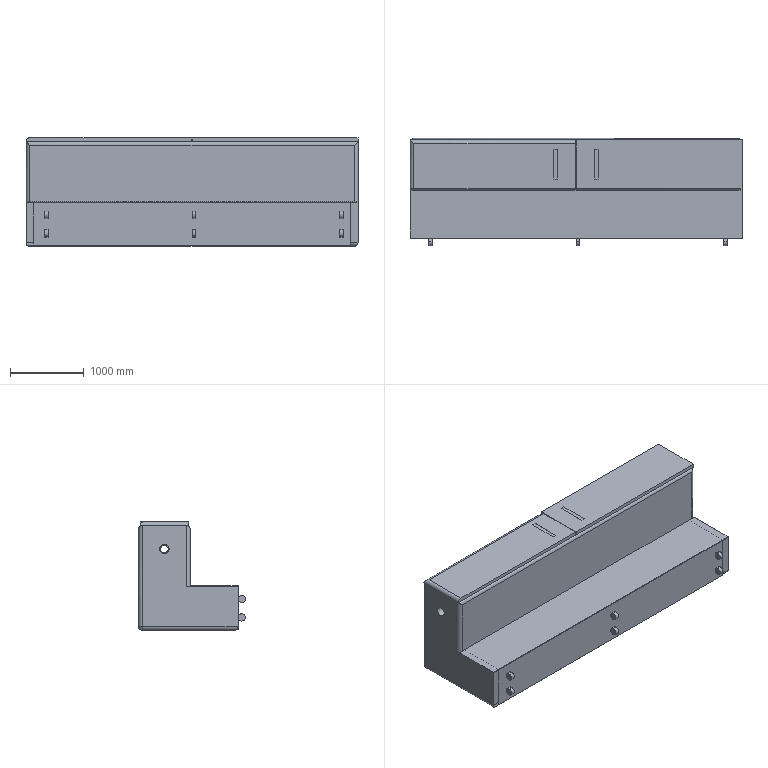Part | SolidWorks | features ICE 13, Cut 2, Fillet 2, LPattern 2, Extrusion 1 | 9 solids | 96 faces | box 4500 x 1450 x 1471 mm | volume 1463085878 mm3 | plane 62 | cylinder 32 | sphere 2 | commonest cylinder face diameters 100 x30 130 x2